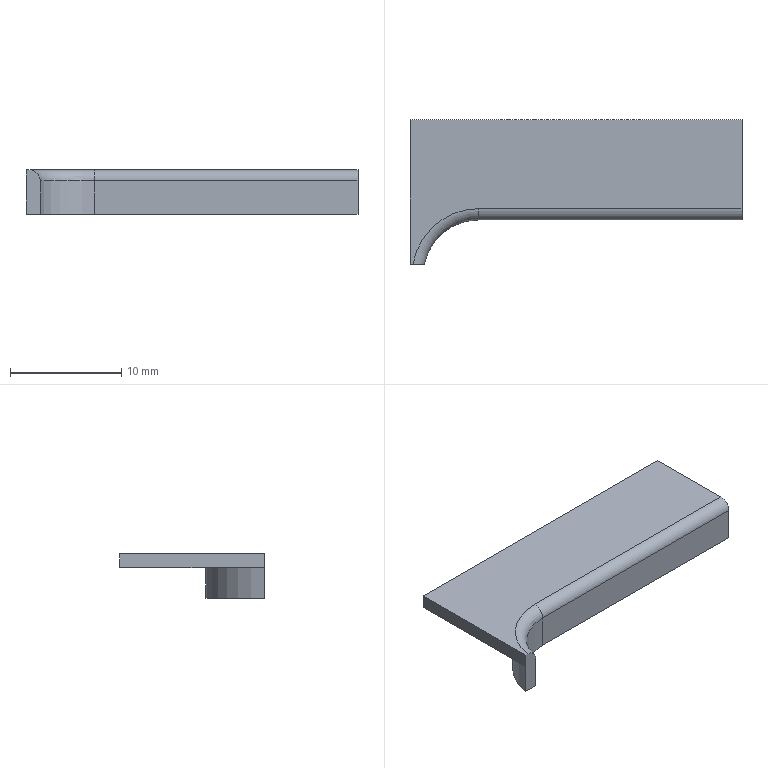Part | STEP file | gslz 2016.10.28-13_id970_x_t | 1 solid | 13 faces | box 29.791 x 13 x 4 mm | volume 449.169 mm3 | plane 9 | cylinder 3 | torus 1 | commonest cylinder face diameters 2 x1 10 x1 12.5 x1
STEP:
#1=CARTESIAN_POINT('',(0.,0.,0.));
#2=DIRECTION('',(0.,0.,1.));
#3=DIRECTION('',(1.,0.,0.));
#4=AXIS2_PLACEMENT_3D('',#1,#2,#3);
#5=CARTESIAN_POINT('',(-716.176,-264.75,0.));
#6=VERTEX_POINT('',#5);
#7=CARTESIAN_POINT('',(-722.345,-270.,0.));
#8=VERTEX_POINT('',#7);
#9=CARTESIAN_POINT('',(-716.176,-271.,0.));
#10=DIRECTION('',(0.,0.,1.));
#11=DIRECTION('',(1.,0.,0.));
#12=AXIS2_PLACEMENT_3D('',#9,#10,#11);
#13=CIRCLE('',#12,6.25);
#14=CARTESIAN_POINT('',(-716.176,-271.,0.625));
#15=DIRECTION('',(0.,0.,1.));
#16=DIRECTION('',(1.,0.,0.));
#17=AXIS2_PLACEMENT_3D('',#14,#15,#16);
#18=CYLINDRICAL_SURFACE('',#17,6.25);
#19=CARTESIAN_POINT('',(0.,-0.625));
#20=DIRECTION('',(1.,0.));
#21=VECTOR('',#20,1.);
#22=LINE('',#19,#21);
#23=(GEOMETRIC_REPRESENTATION_CONTEXT(2)PARAMETRIC_REPRESENTATION_CONTEXT()REPRESENTATION_CONTEXT('',''));
#24=DEFINITIONAL_REPRESENTATION('',(#22),#23);
#25=PCURVE('',#18,#24);
#26=CARTESIAN_POINT('',(1793.591,319.067,0.));
#27=DIRECTION('',(0.,0.,1.));
#28=DIRECTION('',(1.,0.,0.));
#29=AXIS2_PLACEMENT_3D('',#26,#27,#28);
#30=PLANE('',#29);
#31=CARTESIAN_POINT('',(-2509.767,-590.067));
#32=DIRECTION('',(1.,0.));
#33=AXIS2_PLACEMENT_2D('',#31,#32);
#34=CIRCLE('',#33,6.25);
#35=(GEOMETRIC_REPRESENTATION_CONTEXT(2)PARAMETRIC_REPRESENTATION_CONTEXT()REPRESENTATION_CONTEXT('',''));
#36=DEFINITIONAL_REPRESENTATION('',(#34),#35);
#37=PCURVE('',#30,#36);
#38=SURFACE_CURVE('',#13,(#25,#37),.PCURVE_S1.);
#39=EDGE_CURVE('',#6,#8,#38,.T.);
#40=ORIENTED_EDGE('',*,*,#39,.F.);
#41=CARTESIAN_POINT('',(-716.176,-264.75,-2.75));
#42=VERTEX_POINT('',#41);
#43=CARTESIAN_POINT('',(-716.176,-264.75,-0.75));
#44=DIRECTION('',(0.,0.,1.));
#45=VECTOR('',#44,1.);
#46=LINE('',#43,#45);
#47=CARTESIAN_POINT('',(1.571,-1.375));
#48=DIRECTION('',(0.,1.));
#49=VECTOR('',#48,1.);
#50=LINE('',#47,#49);
#51=(GEOMETRIC_REPRESENTATION_CONTEXT(2)PARAMETRIC_REPRESENTATION_CONTEXT()REPRESENTATION_CONTEXT('',''));
#52=DEFINITIONAL_REPRESENTATION('',(#50),#51);
#53=PCURVE('',#18,#52);
#54=CARTESIAN_POINT('',(1463.925,-264.75,-135.834));
#55=DIRECTION('',(0.,-1.,0.));
#56=DIRECTION('',(1.,0.,0.));
#57=AXIS2_PLACEMENT_3D('',#54,#55,#56);
#58=PLANE('',#57);
#59=CARTESIAN_POINT('',(-2180.101,135.084));
#60=DIRECTION('',(0.,1.));
#61=VECTOR('',#60,1.);
#62=LINE('',#59,#61);
#63=(GEOMETRIC_REPRESENTATION_CONTEXT(2)PARAMETRIC_REPRESENTATION_CONTEXT()REPRESENTATION_CONTEXT('',''));
#64=DEFINITIONAL_REPRESENTATION('',(#62),#63);
#65=PCURVE('',#58,#64);
#66=SURFACE_CURVE('',#46,(#53,#65),.PCURVE_S1.);
#67=EDGE_CURVE('',#42,#6,#66,.T.);
#68=ORIENTED_EDGE('',*,*,#67,.F.);
#69=CARTESIAN_POINT('',(-722.345,-270.,-2.75));
#70=VERTEX_POINT('',#69);
#71=CARTESIAN_POINT('',(-716.176,-271.,-2.75));
#72=DIRECTION('',(0.,0.,-1.));
#73=DIRECTION('',(1.,0.,0.));
#74=AXIS2_PLACEMENT_3D('',#71,#72,#73);
#75=CIRCLE('',#74,6.25);
#76=CARTESIAN_POINT('',(6.283,-3.375));
#77=DIRECTION('',(-1.,0.));
#78=VECTOR('',#77,1.);
#79=LINE('',#76,#78);
#80=(GEOMETRIC_REPRESENTATION_CONTEXT(2)PARAMETRIC_REPRESENTATION_CONTEXT()REPRESENTATION_CONTEXT('',''));
#81=DEFINITIONAL_REPRESENTATION('',(#79),#80);
#82=PCURVE('',#18,#81);
#83=CARTESIAN_POINT('',(-1810.,-266.,-2.75));
#84=DIRECTION('',(0.,0.,1.));
#85=DIRECTION('',(-1.,0.,0.));
#86=AXIS2_PLACEMENT_3D('',#83,#84,#85);
#87=PLANE('',#86);
#88=CARTESIAN_POINT('',(-1100.074,5.));
#89=CARTESIAN_POINT('',(-1100.074,15.825));
#90=CARTESIAN_POINT('',(-1090.699,10.413));
#91=CARTESIAN_POINT('',(-1081.324,5.));
#92=CARTESIAN_POINT('',(-1090.699,-0.4127));
#93=CARTESIAN_POINT('',(-1100.074,-5.825));
#94=CARTESIAN_POINT('',(-1100.074,5.));
#95=(BOUNDED_CURVE()B_SPLINE_CURVE(2,(#88,#89,#90,#91,#92,#93,#94),.UNSPECIFIED.,.T.,.F.)B_SPLINE_CURVE_WITH_KNOTS((1,2,2,2,2,1),(-2.094,0.,2.094,4.189,6.283,8.378),.UNSPECIFIED.)CURVE()GEOMETRIC_REPRESENTATION_ITEM()RATIONAL_B_SPLINE_CURVE((1.,0.5,1.,0.5,1.,0.5,1.))REPRESENTATION_ITEM(''));
#96=(GEOMETRIC_REPRESENTATION_CONTEXT(2)PARAMETRIC_REPRESENTATION_CONTEXT()REPRESENTATION_CONTEXT('',''));
#97=DEFINITIONAL_REPRESENTATION('',(#95),#96);
#98=PCURVE('',#87,#97);
#99=SURFACE_CURVE('',#75,(#82,#98),.PCURVE_S1.);
#100=EDGE_CURVE('',#70,#42,#99,.T.);
#101=ORIENTED_EDGE('',*,*,#100,.F.);
#102=CARTESIAN_POINT('',(-722.345,-270.,0.625));
#103=DIRECTION('',(0.,0.,-1.));
#104=VECTOR('',#103,1.);
#105=LINE('',#102,#104);
#106=CARTESIAN_POINT('',(2.981,0.));
#107=DIRECTION('',(0.,-1.));
#108=VECTOR('',#107,1.);
#109=LINE('',#106,#108);
#110=(GEOMETRIC_REPRESENTATION_CONTEXT(2)PARAMETRIC_REPRESENTATION_CONTEXT()REPRESENTATION_CONTEXT('',''));
#111=DEFINITIONAL_REPRESENTATION('',(#109),#110);
#112=PCURVE('',#18,#111);
#113=CARTESIAN_POINT('',(-1810.,-270.,1.25));
#114=DIRECTION('',(0.,1.,0.));
#115=DIRECTION('',(-1.,0.,0.));
#116=AXIS2_PLACEMENT_3D('',#113,#114,#115);
#117=PLANE('',#116);
#118=CARTESIAN_POINT('',(-1087.655,-0.625));
#119=DIRECTION('',(0.,-1.));
#120=VECTOR('',#119,1.);
#121=LINE('',#118,#120);
#122=(GEOMETRIC_REPRESENTATION_CONTEXT(2)PARAMETRIC_REPRESENTATION_CONTEXT()REPRESENTATION_CONTEXT('',''));
#123=DEFINITIONAL_REPRESENTATION('',(#121),#122);
#124=PCURVE('',#117,#123);
#125=SURFACE_CURVE('',#105,(#112,#124),.PCURVE_S1.);
#126=EDGE_CURVE('',#8,#70,#125,.T.);
#127=ORIENTED_EDGE('',*,*,#126,.F.);
#128=EDGE_LOOP('',(#40,#68,#101,#127));
#129=FACE_BOUND('',#128,.T.);
#130=ADVANCED_FACE('',(#129),#18,.T.);
#131=CARTESIAN_POINT('',(-721.075,-270.,-2.75));
#132=VERTEX_POINT('',#131);
#133=CARTESIAN_POINT('',(-721.075,-270.,0.25));
#134=VERTEX_POINT('',#133);
#135=CARTESIAN_POINT('',(-721.075,-270.,61.25));
#136=DIRECTION('',(0.,0.,1.));
#137=VECTOR('',#136,1.);
#138=LINE('',#135,#137);
#139=CARTESIAN_POINT('',(-1088.925,60.));
#140=DIRECTION('',(0.,1.));
#141=VECTOR('',#140,1.);
#142=LINE('',#139,#141);
#143=(GEOMETRIC_REPRESENTATION_CONTEXT(2)PARAMETRIC_REPRESENTATION_CONTEXT()REPRESENTATION_CONTEXT('',''));
#144=DEFINITIONAL_REPRESENTATION('',(#142),#143);
#145=PCURVE('',#117,#144);
#146=CARTESIAN_POINT('',(-716.176,-271.,61.25));
#147=DIRECTION('',(0.,0.,-1.));
#148=DIRECTION('',(-1.,0.,0.));
#149=AXIS2_PLACEMENT_3D('',#146,#147,#148);
#150=CYLINDRICAL_SURFACE('',#149,5.);
#151=CARTESIAN_POINT('',(0.2014,0.));
#152=DIRECTION('',(0.,-1.));
#153=VECTOR('',#152,1.);
#154=LINE('',#151,#153);
#155=(GEOMETRIC_REPRESENTATION_CONTEXT(2)PARAMETRIC_REPRESENTATION_CONTEXT()REPRESENTATION_CONTEXT('',''));
#156=DEFINITIONAL_REPRESENTATION('',(#154),#155);
#157=PCURVE('',#150,#156);
#158=SURFACE_CURVE('',#138,(#145,#157),.PCURVE_S1.);
#159=EDGE_CURVE('',#132,#134,#158,.T.);
#160=ORIENTED_EDGE('',*,*,#159,.T.);
#161=CARTESIAN_POINT('',(-722.092,-270.,1.25));
#162=VERTEX_POINT('',#161);
#163=CARTESIAN_POINT('',(-721.075,-270.,0.25));
#164=CARTESIAN_POINT('',(-721.075,-270.,0.3603));
#165=CARTESIAN_POINT('',(-721.094,-270.,0.4722));
#166=CARTESIAN_POINT('',(-721.131,-270.,0.5763));
#167=CARTESIAN_POINT('',(-721.167,-270.,0.6803));
#168=CARTESIAN_POINT('',(-721.222,-270.,0.7794));
#169=CARTESIAN_POINT('',(-721.291,-270.,0.8657));
#170=CARTESIAN_POINT('',(-721.36,-270.,0.9528));
#171=CARTESIAN_POINT('',(-721.445,-270.,1.029));
#172=CARTESIAN_POINT('',(-721.539,-270.,1.089));
#173=CARTESIAN_POINT('',(-721.635,-270.,1.15));
#174=CARTESIAN_POINT('',(-721.742,-270.,1.196));
#175=CARTESIAN_POINT('',(-721.853,-270.,1.222));
#176=CARTESIAN_POINT('',(-721.931,-270.,1.24));
#177=CARTESIAN_POINT('',(-722.012,-270.,1.25));
#178=CARTESIAN_POINT('',(-722.092,-270.,1.25));
#179=B_SPLINE_CURVE_WITH_KNOTS('',3,(#163,#164,#165,#166,#167,#168,#169,#170,#171,#172,#173,#174,#175,#176,#177,#178),.UNSPECIFIED.,.F.,.F.,(4,3,3,3,3,4),(0.,0.2101,0.4202,0.6322,0.8483,1.),.UNSPECIFIED.);
#180=CARTESIAN_POINT('',(-1088.925,-1.));
#181=CARTESIAN_POINT('',(-1088.925,-0.8897));
#182=CARTESIAN_POINT('',(-1088.906,-0.7778));
#183=CARTESIAN_POINT('',(-1088.869,-0.6737));
#184=CARTESIAN_POINT('',(-1088.833,-0.5697));
#185=CARTESIAN_POINT('',(-1088.778,-0.4706));
#186=CARTESIAN_POINT('',(-1088.709,-0.3843));
#187=CARTESIAN_POINT('',(-1088.64,-0.2972));
#188=CARTESIAN_POINT('',(-1088.555,-0.2207));
#189=CARTESIAN_POINT('',(-1088.461,-0.1609));
#190=CARTESIAN_POINT('',(-1088.365,-0.0999));
#191=CARTESIAN_POINT('',(-1088.258,-0.05448));
#192=CARTESIAN_POINT('',(-1088.147,-0.02814));
#193=CARTESIAN_POINT('',(-1088.069,-0.009512));
#194=CARTESIAN_POINT('',(-1087.988,0.));
#195=CARTESIAN_POINT('',(-1087.908,0.));
#196=B_SPLINE_CURVE_WITH_KNOTS('',3,(#180,#181,#182,#183,#184,#185,#186,#187,#188,#189,#190,#191,#192,#193,#194,#195),.UNSPECIFIED.,.F.,.F.,(4,3,3,3,3,4),(0.,0.2101,0.4202,0.6322,0.8483,1.),.UNSPECIFIED.);
#197=(GEOMETRIC_REPRESENTATION_CONTEXT(2)PARAMETRIC_REPRESENTATION_CONTEXT()REPRESENTATION_CONTEXT('',''));
#198=DEFINITIONAL_REPRESENTATION('',(#196),#197);
#199=PCURVE('',#117,#198);
#200=CARTESIAN_POINT('',(-716.176,-271.,0.25));
#201=DIRECTION('',(0.,0.,1.));
#202=DIRECTION('',(1.,0.,0.));
#203=AXIS2_PLACEMENT_3D('',#200,#201,#202);
#204=TOROIDAL_SURFACE('',#203,6.,1.);
#205=CARTESIAN_POINT('',(2.94,3.142));
#206=CARTESIAN_POINT('',(2.974,1.571));
#207=B_SPLINE_CURVE_WITH_KNOTS('',1,(#205,#206),.UNSPECIFIED.,.F.,.F.,(2,2),(0.,1.),.PIECEWISE_BEZIER_KNOTS.);
#208=(GEOMETRIC_REPRESENTATION_CONTEXT(2)PARAMETRIC_REPRESENTATION_CONTEXT()REPRESENTATION_CONTEXT('',''));
#209=DEFINITIONAL_REPRESENTATION('',(#207),#208);
#210=PCURVE('',#204,#209);
#211=SURFACE_CURVE('',#179,(#199,#210),.PCURVE_S1.);
#212=EDGE_CURVE('',#134,#162,#211,.T.);
#213=ORIENTED_EDGE('',*,*,#212,.T.);
#214=CARTESIAN_POINT('',(-722.345,-270.,1.25));
#215=VERTEX_POINT('',#214);
#216=CARTESIAN_POINT('',(-1810.,-270.,1.25));
#217=DIRECTION('',(-1.,0.,0.));
#218=VECTOR('',#217,1.);
#219=LINE('',#216,#218);
#220=CARTESIAN_POINT('',(0.,0.));
#221=DIRECTION('',(1.,0.));
#222=VECTOR('',#221,1.);
#223=LINE('',#220,#222);
#224=(GEOMETRIC_REPRESENTATION_CONTEXT(2)PARAMETRIC_REPRESENTATION_CONTEXT()REPRESENTATION_CONTEXT('',''));
#225=DEFINITIONAL_REPRESENTATION('',(#223),#224);
#226=PCURVE('',#117,#225);
#227=CARTESIAN_POINT('',(1793.591,319.067,1.25));
#228=DIRECTION('',(0.,0.,1.));
#229=DIRECTION('',(1.,0.,0.));
#230=AXIS2_PLACEMENT_3D('',#227,#228,#229);
#231=PLANE('',#230);
#232=CARTESIAN_POINT('',(-3603.591,-589.067));
#233=DIRECTION('',(-1.,0.));
#234=VECTOR('',#233,1.);
#235=LINE('',#232,#234);
#236=(GEOMETRIC_REPRESENTATION_CONTEXT(2)PARAMETRIC_REPRESENTATION_CONTEXT()REPRESENTATION_CONTEXT('',''));
#237=DEFINITIONAL_REPRESENTATION('',(#235),#236);
#238=PCURVE('',#231,#237);
#239=SURFACE_CURVE('',#219,(#226,#238),.PCURVE_S1.);
#240=EDGE_CURVE('',#162,#215,#239,.T.);
#241=ORIENTED_EDGE('',*,*,#240,.T.);
#242=CARTESIAN_POINT('',(-722.345,-270.,0.625));
#243=DIRECTION('',(0.,0.,-1.));
#244=VECTOR('',#243,1.);
#245=LINE('',#242,#244);
#246=CARTESIAN_POINT('',(-1087.655,-0.625));
#247=DIRECTION('',(0.,-1.));
#248=VECTOR('',#247,1.);
#249=LINE('',#246,#248);
#250=(GEOMETRIC_REPRESENTATION_CONTEXT(2)PARAMETRIC_REPRESENTATION_CONTEXT()REPRESENTATION_CONTEXT('',''));
#251=DEFINITIONAL_REPRESENTATION('',(#249),#250);
#252=PCURVE('',#117,#251);
#253=CARTESIAN_POINT('',(-722.345,-275.25,-0.75));
#254=DIRECTION('',(-1.,0.,0.));
#255=DIRECTION('',(0.,-1.,0.));
#256=AXIS2_PLACEMENT_3D('',#253,#254,#255);
#257=PLANE('',#256);
#258=CARTESIAN_POINT('',(-5.25,1.375));
#259=DIRECTION('',(0.,-1.));
#260=VECTOR('',#259,1.);
#261=LINE('',#258,#260);
#262=(GEOMETRIC_REPRESENTATION_CONTEXT(2)PARAMETRIC_REPRESENTATION_CONTEXT()REPRESENTATION_CONTEXT('',''));
#263=DEFINITIONAL_REPRESENTATION('',(#261),#262);
#264=PCURVE('',#257,#263);
#265=SURFACE_CURVE('',#245,(#252,#264),.PCURVE_S1.);
#266=EDGE_CURVE('',#215,#8,#265,.T.);
#267=ORIENTED_EDGE('',*,*,#266,.T.);
#268=ORIENTED_EDGE('',*,*,#126,.T.);
#269=CARTESIAN_POINT('',(-1810.,-270.,-2.75));
#270=DIRECTION('',(1.,0.,0.));
#271=VECTOR('',#270,1.);
#272=LINE('',#269,#271);
#273=CARTESIAN_POINT('',(0.,-4.));
#274=DIRECTION('',(-1.,0.));
#275=VECTOR('',#274,1.);
#276=LINE('',#273,#275);
#277=(GEOMETRIC_REPRESENTATION_CONTEXT(2)PARAMETRIC_REPRESENTATION_CONTEXT()REPRESENTATION_CONTEXT('',''));
#278=DEFINITIONAL_REPRESENTATION('',(#276),#277);
#279=PCURVE('',#117,#278);
#280=CARTESIAN_POINT('',(0.,4.));
#281=DIRECTION('',(-1.,0.));
#282=VECTOR('',#281,1.);
#283=LINE('',#280,#282);
#284=(GEOMETRIC_REPRESENTATION_CONTEXT(2)PARAMETRIC_REPRESENTATION_CONTEXT()REPRESENTATION_CONTEXT('',''));
#285=DEFINITIONAL_REPRESENTATION('',(#283),#284);
#286=PCURVE('',#87,#285);
#287=SURFACE_CURVE('',#272,(#279,#286),.PCURVE_S1.);
#288=EDGE_CURVE('',#70,#132,#287,.T.);
#289=ORIENTED_EDGE('',*,*,#288,.T.);
#290=EDGE_LOOP('',(#160,#213,#241,#267,#268,#289));
#291=FACE_BOUND('',#290,.T.);
#292=ADVANCED_FACE('',(#291),#117,.F.);
#293=CARTESIAN_POINT('',(-716.176,-266.,-2.75));
#294=VERTEX_POINT('',#293);
#295=CARTESIAN_POINT('',(-716.176,-271.,-2.75));
#296=DIRECTION('',(0.,0.,1.));
#297=DIRECTION('',(1.,0.,0.));
#298=AXIS2_PLACEMENT_3D('',#295,#296,#297);
#299=CIRCLE('',#298,5.);
#300=CARTESIAN_POINT('',(3.142,64.));
#301=DIRECTION('',(-1.,0.));
#302=VECTOR('',#301,1.);
#303=LINE('',#300,#302);
#304=(GEOMETRIC_REPRESENTATION_CONTEXT(2)PARAMETRIC_REPRESENTATION_CONTEXT()REPRESENTATION_CONTEXT('',''));
#305=DEFINITIONAL_REPRESENTATION('',(#303),#304);
#306=PCURVE('',#150,#305);
#307=CARTESIAN_POINT('',(-1093.824,5.));
#308=DIRECTION('',(-1.,0.));
#309=AXIS2_PLACEMENT_2D('',#307,#308);
#310=CIRCLE('',#309,5.);
#311=(GEOMETRIC_REPRESENTATION_CONTEXT(2)PARAMETRIC_REPRESENTATION_CONTEXT()REPRESENTATION_CONTEXT('',''));
#312=DEFINITIONAL_REPRESENTATION('',(#310),#311);
#313=PCURVE('',#87,#312);
#314=SURFACE_CURVE('',#299,(#306,#313),.PCURVE_S1.);
#315=EDGE_CURVE('',#294,#132,#314,.T.);
#316=ORIENTED_EDGE('',*,*,#315,.T.);
#317=ORIENTED_EDGE('',*,*,#159,.T.);
#318=CARTESIAN_POINT('',(-716.176,-266.,0.25));
#319=VERTEX_POINT('',#318);
#320=CARTESIAN_POINT('',(-716.176,-271.,0.25));
#321=DIRECTION('',(0.,0.,1.));
#322=DIRECTION('',(1.,0.,0.));
#323=AXIS2_PLACEMENT_3D('',#320,#321,#322);
#324=CIRCLE('',#323,5.);
#325=CARTESIAN_POINT('',(3.142,61.));
#326=DIRECTION('',(-1.,0.));
#327=VECTOR('',#326,1.);
#328=LINE('',#325,#327);
#329=(GEOMETRIC_REPRESENTATION_CONTEXT(2)PARAMETRIC_REPRESENTATION_CONTEXT()REPRESENTATION_CONTEXT('',''));
#330=DEFINITIONAL_REPRESENTATION('',(#328),#329);
#331=PCURVE('',#150,#330);
#332=CARTESIAN_POINT('',(0.,3.142));
#333=DIRECTION('',(1.,0.));
#334=VECTOR('',#333,1.);
#335=LINE('',#332,#334);
#336=(GEOMETRIC_REPRESENTATION_CONTEXT(2)PARAMETRIC_REPRESENTATION_CONTEXT()REPRESENTATION_CONTEXT('',''));
#337=DEFINITIONAL_REPRESENTATION('',(#335),#336);
#338=PCURVE('',#204,#337);
#339=SURFACE_CURVE('',#324,(#331,#338),.PCURVE_S1.);
#340=EDGE_CURVE('',#319,#134,#339,.T.);
#341=ORIENTED_EDGE('',*,*,#340,.F.);
#342=CARTESIAN_POINT('',(-716.176,-266.,61.25));
#343=DIRECTION('',(0.,0.,-1.));
#344=VECTOR('',#343,1.);
#345=LINE('',#342,#344);
#346=CARTESIAN_POINT('',(1.571,0.));
#347=DIRECTION('',(0.,1.));
#348=VECTOR('',#347,1.);
#349=LINE('',#346,#348);
#350=(GEOMETRIC_REPRESENTATION_CONTEXT(2)PARAMETRIC_REPRESENTATION_CONTEXT()REPRESENTATION_CONTEXT('',''));
#351=DEFINITIONAL_REPRESENTATION('',(#349),#350);
#352=PCURVE('',#150,#351);
#353=CARTESIAN_POINT('',(-548.575,-266.,0.625));
#354=DIRECTION('',(0.,-1.,0.));
#355=DIRECTION('',(1.,0.,0.));
#356=AXIS2_PLACEMENT_3D('',#353,#354,#355);
#357=PLANE('',#356);
#358=CARTESIAN_POINT('',(-167.601,60.625));
#359=DIRECTION('',(0.,-1.));
#360=VECTOR('',#359,1.);
#361=LINE('',#358,#360);
#362=(GEOMETRIC_REPRESENTATION_CONTEXT(2)PARAMETRIC_REPRESENTATION_CONTEXT()REPRESENTATION_CONTEXT('',''));
#363=DEFINITIONAL_REPRESENTATION('',(#361),#362);
#364=PCURVE('',#357,#363);
#365=SURFACE_CURVE('',#345,(#352,#364),.PCURVE_S1.);
#366=EDGE_CURVE('',#319,#294,#365,.T.);
#367=ORIENTED_EDGE('',*,*,#366,.T.);
#368=EDGE_LOOP('',(#316,#317,#341,#367));
#369=FACE_BOUND('',#368,.F.);
#370=ADVANCED_FACE('',(#369),#150,.F.);
#371=ORIENTED_EDGE('',*,*,#212,.F.);
#372=ORIENTED_EDGE('',*,*,#340,.F.);
#373=CARTESIAN_POINT('',(-716.176,-265.,1.25));
#374=VERTEX_POINT('',#373);
#375=CARTESIAN_POINT('',(-716.176,-265.,0.25));
#376=DIRECTION('',(1.,0.,0.));
#377=DIRECTION('',(0.,0.,-1.));
#378=AXIS2_PLACEMENT_3D('',#375,#376,#377);
#379=CIRCLE('',#378,1.);
#380=CARTESIAN_POINT('',(1.571,-1.571));
#381=DIRECTION('',(0.,1.));
#382=VECTOR('',#381,1.);
#383=LINE('',#380,#382);
#384=(GEOMETRIC_REPRESENTATION_CONTEXT(2)PARAMETRIC_REPRESENTATION_CONTEXT()REPRESENTATION_CONTEXT('',''));
#385=DEFINITIONAL_REPRESENTATION('',(#383),#384);
#386=PCURVE('',#204,#385);
#387=CARTESIAN_POINT('',(1793.591,-265.,0.25));
#388=DIRECTION('',(1.,0.,0.));
#389=DIRECTION('',(0.,1.,0.));
#390=AXIS2_PLACEMENT_3D('',#387,#388,#389);
#391=CYLINDRICAL_SURFACE('',#390,1.);
#392=CARTESIAN_POINT('',(-1.571,-2509.767));
#393=DIRECTION('',(1.,0.));
#394=VECTOR('',#393,1.);
#395=LINE('',#392,#394);
#396=(GEOMETRIC_REPRESENTATION_CONTEXT(2)PARAMETRIC_REPRESENTATION_CONTEXT()REPRESENTATION_CONTEXT('',''));
#397=DEFINITIONAL_REPRESENTATION('',(#395),#396);
#398=PCURVE('',#391,#397);
#399=SURFACE_CURVE('',#379,(#386,#398),.PCURVE_S1.);
#400=EDGE_CURVE('',#374,#319,#399,.T.);
#401=ORIENTED_EDGE('',*,*,#400,.F.);
#402=CARTESIAN_POINT('',(-716.176,-271.,1.25));
#403=DIRECTION('',(0.,0.,-1.));
#404=DIRECTION('',(1.,0.,0.));
#405=AXIS2_PLACEMENT_3D('',#402,#403,#404);
#406=CIRCLE('',#405,6.);
#407=CARTESIAN_POINT('',(6.283,1.571));
#408=DIRECTION('',(-1.,0.));
#409=VECTOR('',#408,1.);
#410=LINE('',#407,#409);
#411=(GEOMETRIC_REPRESENTATION_CONTEXT(2)PARAMETRIC_REPRESENTATION_CONTEXT()REPRESENTATION_CONTEXT('',''));
#412=DEFINITIONAL_REPRESENTATION('',(#410),#411);
#413=PCURVE('',#204,#412);
#414=CARTESIAN_POINT('',(-2503.767,-590.067));
#415=CARTESIAN_POINT('',(-2503.767,-600.459));
#416=CARTESIAN_POINT('',(-2512.767,-595.263));
#417=CARTESIAN_POINT('',(-2521.767,-590.067));
#418=CARTESIAN_POINT('',(-2512.767,-584.871));
#419=CARTESIAN_POINT('',(-2503.767,-579.674));
#420=CARTESIAN_POINT('',(-2503.767,-590.067));
#421=(BOUNDED_CURVE()B_SPLINE_CURVE(2,(#414,#415,#416,#417,#418,#419,#420),.UNSPECIFIED.,.T.,.F.)B_SPLINE_CURVE_WITH_KNOTS((1,2,2,2,2,1),(-2.094,0.,2.094,4.189,6.283,8.378),.UNSPECIFIED.)CURVE()GEOMETRIC_REPRESENTATION_ITEM()RATIONAL_B_SPLINE_CURVE((1.,0.5,1.,0.5,1.,0.5,1.))REPRESENTATION_ITEM(''));
#422=(GEOMETRIC_REPRESENTATION_CONTEXT(2)PARAMETRIC_REPRESENTATION_CONTEXT()REPRESENTATION_CONTEXT('',''));
#423=DEFINITIONAL_REPRESENTATION('',(#421),#422);
#424=PCURVE('',#231,#423);
#425=SURFACE_CURVE('',#406,(#413,#424),.PCURVE_S1.);
#426=EDGE_CURVE('',#162,#374,#425,.T.);
#427=ORIENTED_EDGE('',*,*,#426,.F.);
#428=EDGE_LOOP('',(#371,#372,#401,#427));
#429=FACE_BOUND('',#428,.T.);
#430=ADVANCED_FACE('',(#429),#204,.T.);
#431=CARTESIAN_POINT('',(-722.345,-257.,1.25));
#432=VERTEX_POINT('',#431);
#433=CARTESIAN_POINT('',(-722.345,319.067,1.25));
#434=DIRECTION('',(0.,1.,0.));
#435=VECTOR('',#434,1.);
#436=LINE('',#433,#435);
#437=CARTESIAN_POINT('',(-594.317,2.));
#438=DIRECTION('',(-1.,0.));
#439=VECTOR('',#438,1.);
#440=LINE('',#437,#439);
#441=(GEOMETRIC_REPRESENTATION_CONTEXT(2)PARAMETRIC_REPRESENTATION_CONTEXT()REPRESENTATION_CONTEXT('',''));
#442=DEFINITIONAL_REPRESENTATION('',(#440),#441);
#443=PCURVE('',#257,#442);
#444=CARTESIAN_POINT('',(-2515.936,0.));
#445=DIRECTION('',(0.,1.));
#446=VECTOR('',#445,1.);
#447=LINE('',#444,#446);
#448=(GEOMETRIC_REPRESENTATION_CONTEXT(2)PARAMETRIC_REPRESENTATION_CONTEXT()REPRESENTATION_CONTEXT('',''));
#449=DEFINITIONAL_REPRESENTATION('',(#447),#448);
#450=PCURVE('',#231,#449);
#451=SURFACE_CURVE('',#436,(#443,#450),.PCURVE_S1.);
#452=EDGE_CURVE('',#215,#432,#451,.T.);
#453=ORIENTED_EDGE('',*,*,#452,.T.);
#454=CARTESIAN_POINT('',(-722.345,-257.,0.));
#455=VERTEX_POINT('',#454);
#456=CARTESIAN_POINT('',(-722.345,-257.,2.5));
#457=DIRECTION('',(0.,0.,1.));
#458=VECTOR('',#457,1.);
#459=LINE('',#456,#458);
#460=CARTESIAN_POINT('',(-18.25,3.25));
#461=DIRECTION('',(0.,1.));
#462=VECTOR('',#461,1.);
#463=LINE('',#460,#462);
#464=(GEOMETRIC_REPRESENTATION_CONTEXT(2)PARAMETRIC_REPRESENTATION_CONTEXT()REPRESENTATION_CONTEXT('',''));
#465=DEFINITIONAL_REPRESENTATION('',(#463),#464);
#466=PCURVE('',#257,#465);
#467=CARTESIAN_POINT('',(-705.557,-257.,2.5));
#468=DIRECTION('',(0.,1.,0.));
#469=DIRECTION('',(0.,0.,1.));
#470=AXIS2_PLACEMENT_3D('',#467,#468,#469);
#471=PLANE('',#470);
#472=CARTESIAN_POINT('',(0.,-16.788));
#473=DIRECTION('',(1.,0.));
#474=VECTOR('',#473,1.);
#475=LINE('',#472,#474);
#476=(GEOMETRIC_REPRESENTATION_CONTEXT(2)PARAMETRIC_REPRESENTATION_CONTEXT()REPRESENTATION_CONTEXT('',''));
#477=DEFINITIONAL_REPRESENTATION('',(#475),#476);
#478=PCURVE('',#471,#477);
#479=SURFACE_CURVE('',#459,(#466,#478),.PCURVE_S1.);
#480=EDGE_CURVE('',#455,#432,#479,.T.);
#481=ORIENTED_EDGE('',*,*,#480,.F.);
#482=CARTESIAN_POINT('',(-722.345,319.067,0.));
#483=DIRECTION('',(0.,1.,0.));
#484=VECTOR('',#483,1.);
#485=LINE('',#482,#484);
#486=CARTESIAN_POINT('',(-594.317,0.75));
#487=DIRECTION('',(-1.,0.));
#488=VECTOR('',#487,1.);
#489=LINE('',#486,#488);
#490=(GEOMETRIC_REPRESENTATION_CONTEXT(2)PARAMETRIC_REPRESENTATION_CONTEXT()REPRESENTATION_CONTEXT('',''));
#491=DEFINITIONAL_REPRESENTATION('',(#489),#490);
#492=PCURVE('',#257,#491);
#493=CARTESIAN_POINT('',(-2515.936,0.));
#494=DIRECTION('',(0.,1.));
#495=VECTOR('',#494,1.);
#496=LINE('',#493,#495);
#497=(GEOMETRIC_REPRESENTATION_CONTEXT(2)PARAMETRIC_REPRESENTATION_CONTEXT()REPRESENTATION_CONTEXT('',''));
#498=DEFINITIONAL_REPRESENTATION('',(#496),#497);
#499=PCURVE('',#30,#498);
#500=SURFACE_CURVE('',#485,(#492,#499),.PCURVE_S1.);
#501=EDGE_CURVE('',#8,#455,#500,.T.);
#502=ORIENTED_EDGE('',*,*,#501,.F.);
#503=ORIENTED_EDGE('',*,*,#266,.F.);
#504=EDGE_LOOP('',(#453,#481,#502,#503));
#505=FACE_BOUND('',#504,.T.);
#506=ADVANCED_FACE('',(#505),#257,.T.);
#507=CARTESIAN_POINT('',(-692.554,-266.,0.25));
#508=VERTEX_POINT('',#507);
#509=CARTESIAN_POINT('',(-692.554,-265.,1.25));
#510=VERTEX_POINT('',#509);
#511=CARTESIAN_POINT('',(-692.554,-265.,0.25));
#512=DIRECTION('',(-1.,0.,0.));
#513=DIRECTION('',(0.,0.,1.));
#514=AXIS2_PLACEMENT_3D('',#511,#512,#513);
#515=CIRCLE('',#514,1.);
#516=CARTESIAN_POINT('',(7.854,-2486.145));
#517=DIRECTION('',(-1.,0.));
#518=VECTOR('',#517,1.);
#519=LINE('',#516,#518);
#520=(GEOMETRIC_REPRESENTATION_CONTEXT(2)PARAMETRIC_REPRESENTATION_CONTEXT()REPRESENTATION_CONTEXT('',''));
#521=DEFINITIONAL_REPRESENTATION('',(#519),#520);
#522=PCURVE('',#391,#521);
#523=CARTESIAN_POINT('',(-692.554,-244.358,-2.25));
#524=DIRECTION('',(-1.,0.,0.));
#525=DIRECTION('',(0.,0.,1.));
#526=AXIS2_PLACEMENT_3D('',#523,#524,#525);
#527=PLANE('',#526);
#528=CARTESIAN_POINT('',(2.5,-20.642));
#529=DIRECTION('',(1.,0.));
#530=AXIS2_PLACEMENT_2D('',#528,#529);
#531=CIRCLE('',#530,1.);
#532=(GEOMETRIC_REPRESENTATION_CONTEXT(2)PARAMETRIC_REPRESENTATION_CONTEXT()REPRESENTATION_CONTEXT('',''));
#533=DEFINITIONAL_REPRESENTATION('',(#531),#532);
#534=PCURVE('',#527,#533);
#535=SURFACE_CURVE('',#515,(#522,#534),.PCURVE_S1.);
#536=EDGE_CURVE('',#508,#510,#535,.T.);
#537=ORIENTED_EDGE('',*,*,#536,.T.);
#538=CARTESIAN_POINT('',(1793.591,-265.,1.25));
#539=DIRECTION('',(1.,0.,0.));
#540=VECTOR('',#539,1.);
#541=LINE('',#538,#540);
#542=CARTESIAN_POINT('',(1.571,0.));
#543=DIRECTION('',(0.,1.));
#544=VECTOR('',#543,1.);
#545=LINE('',#542,#544);
#546=(GEOMETRIC_REPRESENTATION_CONTEXT(2)PARAMETRIC_REPRESENTATION_CONTEXT()REPRESENTATION_CONTEXT('',''));
#547=DEFINITIONAL_REPRESENTATION('',(#545),#546);
#548=PCURVE('',#391,#547);
#549=CARTESIAN_POINT('',(0.,-584.067));
#550=DIRECTION('',(1.,0.));
#551=VECTOR('',#550,1.);
#552=LINE('',#549,#551);
#553=(GEOMETRIC_REPRESENTATION_CONTEXT(2)PARAMETRIC_REPRESENTATION_CONTEXT()REPRESENTATION_CONTEXT('',''));
#554=DEFINITIONAL_REPRESENTATION('',(#552),#553);
#555=PCURVE('',#231,#554);
#556=SURFACE_CURVE('',#541,(#548,#555),.PCURVE_S1.);
#557=EDGE_CURVE('',#374,#510,#556,.T.);
#558=ORIENTED_EDGE('',*,*,#557,.F.);
#559=ORIENTED_EDGE('',*,*,#400,.T.);
#560=CARTESIAN_POINT('',(-548.575,-266.,0.25));
#561=DIRECTION('',(-1.,0.,0.));
#562=VECTOR('',#561,1.);
#563=LINE('',#560,#562);
#564=CARTESIAN_POINT('',(3.142,-2342.166));
#565=DIRECTION('',(0.,-1.));
#566=VECTOR('',#565,1.);
#567=LINE('',#564,#566);
#568=(GEOMETRIC_REPRESENTATION_CONTEXT(2)PARAMETRIC_REPRESENTATION_CONTEXT()REPRESENTATION_CONTEXT('',''));
#569=DEFINITIONAL_REPRESENTATION('',(#567),#568);
#570=PCURVE('',#391,#569);
#571=CARTESIAN_POINT('',(0.,-0.375));
#572=DIRECTION('',(-1.,0.));
#573=VECTOR('',#572,1.);
#574=LINE('',#571,#573);
#575=(GEOMETRIC_REPRESENTATION_CONTEXT(2)PARAMETRIC_REPRESENTATION_CONTEXT()REPRESENTATION_CONTEXT('',''));
#576=DEFINITIONAL_REPRESENTATION('',(#574),#575);
#577=PCURVE('',#357,#576);
#578=SURFACE_CURVE('',#563,(#570,#577),.PCURVE_S1.);
#579=EDGE_CURVE('',#508,#319,#578,.T.);
#580=ORIENTED_EDGE('',*,*,#579,.F.);
#581=EDGE_LOOP('',(#537,#558,#559,#580));
#582=FACE_BOUND('',#581,.T.);
#583=ADVANCED_FACE('',(#582),#391,.T.);
#584=CARTESIAN_POINT('',(-692.554,-266.,-2.75));
#585=VERTEX_POINT('',#584);
#586=CARTESIAN_POINT('',(-692.554,-266.,0.625));
#587=DIRECTION('',(0.,0.,1.));
#588=VECTOR('',#587,1.);
#589=LINE('',#586,#588);
#590=CARTESIAN_POINT('',(-143.979,0.));
#591=DIRECTION('',(0.,1.));
#592=VECTOR('',#591,1.);
#593=LINE('',#590,#592);
#594=(GEOMETRIC_REPRESENTATION_CONTEXT(2)PARAMETRIC_REPRESENTATION_CONTEXT()REPRESENTATION_CONTEXT('',''));
#595=DEFINITIONAL_REPRESENTATION('',(#593),#594);
#596=PCURVE('',#357,#595);
#597=CARTESIAN_POINT('',(2.875,-21.642));
#598=DIRECTION('',(1.,0.));
#599=VECTOR('',#598,1.);
#600=LINE('',#597,#599);
#601=(GEOMETRIC_REPRESENTATION_CONTEXT(2)PARAMETRIC_REPRESENTATION_CONTEXT()REPRESENTATION_CONTEXT('',''));
#602=DEFINITIONAL_REPRESENTATION('',(#600),#601);
#603=PCURVE('',#527,#602);
#604=SURFACE_CURVE('',#589,(#596,#603),.PCURVE_S1.);
#605=EDGE_CURVE('',#585,#508,#604,.T.);
#606=ORIENTED_EDGE('',*,*,#605,.T.);
#607=ORIENTED_EDGE('',*,*,#579,.T.);
#608=ORIENTED_EDGE('',*,*,#366,.T.);
#609=CARTESIAN_POINT('',(-1810.,-266.,-2.75));
#610=DIRECTION('',(-1.,0.,0.));
#611=VECTOR('',#610,1.);
#612=LINE('',#609,#611);
#613=CARTESIAN_POINT('',(-1261.425,-3.375));
#614=DIRECTION('',(-1.,0.));
#615=VECTOR('',#614,1.);
#616=LINE('',#613,#615);
#617=(GEOMETRIC_REPRESENTATION_CONTEXT(2)PARAMETRIC_REPRESENTATION_CONTEXT()REPRESENTATION_CONTEXT('',''));
#618=DEFINITIONAL_REPRESENTATION('',(#616),#617);
#619=PCURVE('',#357,#618);
#620=CARTESIAN_POINT('',(0.,0.));
#621=DIRECTION('',(1.,0.));
#622=VECTOR('',#621,1.);
#623=LINE('',#620,#622);
#624=(GEOMETRIC_REPRESENTATION_CONTEXT(2)PARAMETRIC_REPRESENTATION_CONTEXT()REPRESENTATION_CONTEXT('',''));
#625=DEFINITIONAL_REPRESENTATION('',(#623),#624);
#626=PCURVE('',#87,#625);
#627=SURFACE_CURVE('',#612,(#619,#626),.PCURVE_S1.);
#628=EDGE_CURVE('',#585,#294,#627,.T.);
#629=ORIENTED_EDGE('',*,*,#628,.F.);
#630=EDGE_LOOP('',(#606,#607,#608,#629));
#631=FACE_BOUND('',#630,.T.);
#632=ADVANCED_FACE('',(#631),#357,.T.);
#633=CARTESIAN_POINT('',(-692.554,-264.75,-2.75));
#634=VERTEX_POINT('',#633);
#635=CARTESIAN_POINT('',(-1810.,-264.75,-2.75));
#636=DIRECTION('',(-1.,0.,0.));
#637=VECTOR('',#636,1.);
#638=LINE('',#635,#637);
#639=CARTESIAN_POINT('',(0.,-1.25));
#640=DIRECTION('',(1.,0.));
#641=VECTOR('',#640,1.);
#642=LINE('',#639,#641);
#643=(GEOMETRIC_REPRESENTATION_CONTEXT(2)PARAMETRIC_REPRESENTATION_CONTEXT()REPRESENTATION_CONTEXT('',''));
#644=DEFINITIONAL_REPRESENTATION('',(#642),#643);
#645=PCURVE('',#87,#644);
#646=CARTESIAN_POINT('',(-3273.925,133.084));
#647=DIRECTION('',(-1.,0.));
#648=VECTOR('',#647,1.);
#649=LINE('',#646,#648);
#650=(GEOMETRIC_REPRESENTATION_CONTEXT(2)PARAMETRIC_REPRESENTATION_CONTEXT()REPRESENTATION_CONTEXT('',''));
#651=DEFINITIONAL_REPRESENTATION('',(#649),#650);
#652=PCURVE('',#58,#651);
#653=SURFACE_CURVE('',#638,(#645,#652),.PCURVE_S1.);
#654=EDGE_CURVE('',#634,#42,#653,.T.);
#655=ORIENTED_EDGE('',*,*,#654,.F.);
#656=CARTESIAN_POINT('',(-692.554,-266.,-2.75));
#657=DIRECTION('',(0.,-1.,0.));
#658=VECTOR('',#657,1.);
#659=LINE('',#656,#658);
#660=CARTESIAN_POINT('',(-1117.446,0.));
#661=DIRECTION('',(0.,1.));
#662=VECTOR('',#661,1.);
#663=LINE('',#660,#662);
#664=(GEOMETRIC_REPRESENTATION_CONTEXT(2)PARAMETRIC_REPRESENTATION_CONTEXT()REPRESENTATION_CONTEXT('',''));
#665=DEFINITIONAL_REPRESENTATION('',(#663),#664);
#666=PCURVE('',#87,#665);
#667=CARTESIAN_POINT('',(-0.5,-21.642));
#668=DIRECTION('',(0.,-1.));
#669=VECTOR('',#668,1.);
#670=LINE('',#667,#669);
#671=(GEOMETRIC_REPRESENTATION_CONTEXT(2)PARAMETRIC_REPRESENTATION_CONTEXT()REPRESENTATION_CONTEXT('',''));
#672=DEFINITIONAL_REPRESENTATION('',(#670),#671);
#673=PCURVE('',#527,#672);
#674=SURFACE_CURVE('',#659,(#666,#673),.PCURVE_S1.);
#675=EDGE_CURVE('',#634,#585,#674,.T.);
#676=ORIENTED_EDGE('',*,*,#675,.T.);
#677=ORIENTED_EDGE('',*,*,#628,.T.);
#678=ORIENTED_EDGE('',*,*,#315,.T.);
#679=ORIENTED_EDGE('',*,*,#288,.F.);
#680=ORIENTED_EDGE('',*,*,#100,.T.);
#681=EDGE_LOOP('',(#655,#676,#677,#678,#679,#680));
#682=FACE_BOUND('',#681,.T.);
#683=ADVANCED_FACE('',(#682),#87,.F.);
#684=CARTESIAN_POINT('',(-692.554,-264.75,0.));
#685=VERTEX_POINT('',#684);
#686=CARTESIAN_POINT('',(1793.591,-264.75,0.));
#687=DIRECTION('',(1.,0.,0.));
#688=VECTOR('',#687,1.);
#689=LINE('',#686,#688);
#690=CARTESIAN_POINT('',(329.666,135.834));
#691=DIRECTION('',(1.,0.));
#692=VECTOR('',#691,1.);
#693=LINE('',#690,#692);
#694=(GEOMETRIC_REPRESENTATION_CONTEXT(2)PARAMETRIC_REPRESENTATION_CONTEXT()REPRESENTATION_CONTEXT('',''));
#695=DEFINITIONAL_REPRESENTATION('',(#693),#694);
#696=PCURVE('',#58,#695);
#697=CARTESIAN_POINT('',(0.,-583.817));
#698=DIRECTION('',(1.,0.));
#699=VECTOR('',#698,1.);
#700=LINE('',#697,#699);
#701=(GEOMETRIC_REPRESENTATION_CONTEXT(2)PARAMETRIC_REPRESENTATION_CONTEXT()REPRESENTATION_CONTEXT('',''));
#702=DEFINITIONAL_REPRESENTATION('',(#700),#701);
#703=PCURVE('',#30,#702);
#704=SURFACE_CURVE('',#689,(#696,#703),.PCURVE_S1.);
#705=EDGE_CURVE('',#6,#685,#704,.T.);
#706=ORIENTED_EDGE('',*,*,#705,.T.);
#707=CARTESIAN_POINT('',(-692.554,-264.75,-135.834));
#708=DIRECTION('',(0.,0.,-1.));
#709=VECTOR('',#708,1.);
#710=LINE('',#707,#709);
#711=CARTESIAN_POINT('',(-2156.479,0.));
#712=DIRECTION('',(0.,-1.));
#713=VECTOR('',#712,1.);
#714=LINE('',#711,#713);
#715=(GEOMETRIC_REPRESENTATION_CONTEXT(2)PARAMETRIC_REPRESENTATION_CONTEXT()REPRESENTATION_CONTEXT('',''));
#716=DEFINITIONAL_REPRESENTATION('',(#714),#715);
#717=PCURVE('',#58,#716);
#718=CARTESIAN_POINT('',(-133.584,-20.392));
#719=DIRECTION('',(-1.,0.));
#720=VECTOR('',#719,1.);
#721=LINE('',#718,#720);
#722=(GEOMETRIC_REPRESENTATION_CONTEXT(2)PARAMETRIC_REPRESENTATION_CONTEXT()REPRESENTATION_CONTEXT('',''));
#723=DEFINITIONAL_REPRESENTATION('',(#721),#722);
#724=PCURVE('',#527,#723);
#725=SURFACE_CURVE('',#710,(#717,#724),.PCURVE_S1.);
#726=EDGE_CURVE('',#685,#634,#725,.T.);
#727=ORIENTED_EDGE('',*,*,#726,.T.);
#728=ORIENTED_EDGE('',*,*,#654,.T.);
#729=ORIENTED_EDGE('',*,*,#67,.T.);
#730=EDGE_LOOP('',(#706,#727,#728,#729));
#731=FACE_BOUND('',#730,.T.);
#732=ADVANCED_FACE('',(#731),#58,.F.);
#733=CARTESIAN_POINT('',(-692.554,-257.,0.));
#734=VERTEX_POINT('',#733);
#735=CARTESIAN_POINT('',(-692.554,-257.,1.25));
#736=VERTEX_POINT('',#735);
#737=CARTESIAN_POINT('',(-692.554,-257.,2.5));
#738=DIRECTION('',(0.,0.,1.));
#739=VECTOR('',#738,1.);
#740=LINE('',#737,#739);
#741=CARTESIAN_POINT('',(0.,13.004));
#742=DIRECTION('',(1.,0.));
#743=VECTOR('',#742,1.);
#744=LINE('',#741,#743);
#745=(GEOMETRIC_REPRESENTATION_CONTEXT(2)PARAMETRIC_REPRESENTATION_CONTEXT()REPRESENTATION_CONTEXT('',''));
#746=DEFINITIONAL_REPRESENTATION('',(#744),#745);
#747=PCURVE('',#471,#746);
#748=CARTESIAN_POINT('',(4.75,-12.642));
#749=DIRECTION('',(1.,0.));
#750=VECTOR('',#749,1.);
#751=LINE('',#748,#750);
#752=(GEOMETRIC_REPRESENTATION_CONTEXT(2)PARAMETRIC_REPRESENTATION_CONTEXT()REPRESENTATION_CONTEXT('',''));
#753=DEFINITIONAL_REPRESENTATION('',(#751),#752);
#754=PCURVE('',#527,#753);
#755=SURFACE_CURVE('',#740,(#747,#754),.PCURVE_S1.);
#756=EDGE_CURVE('',#734,#736,#755,.T.);
#757=ORIENTED_EDGE('',*,*,#756,.F.);
#758=CARTESIAN_POINT('',(-705.557,-257.,0.));
#759=DIRECTION('',(1.,0.,0.));
#760=VECTOR('',#759,1.);
#761=LINE('',#758,#760);
#762=CARTESIAN_POINT('',(-2.5,0.));
#763=DIRECTION('',(0.,1.));
#764=VECTOR('',#763,1.);
#765=LINE('',#762,#764);
#766=(GEOMETRIC_REPRESENTATION_CONTEXT(2)PARAMETRIC_REPRESENTATION_CONTEXT()REPRESENTATION_CONTEXT('',''));
#767=DEFINITIONAL_REPRESENTATION('',(#765),#766);
#768=PCURVE('',#471,#767);
#769=CARTESIAN_POINT('',(-2499.149,-576.067));
#770=DIRECTION('',(1.,0.));
#771=VECTOR('',#770,1.);
#772=LINE('',#769,#771);
#773=(GEOMETRIC_REPRESENTATION_CONTEXT(2)PARAMETRIC_REPRESENTATION_CONTEXT()REPRESENTATION_CONTEXT('',''));
#774=DEFINITIONAL_REPRESENTATION('',(#772),#773);
#775=PCURVE('',#30,#774);
#776=SURFACE_CURVE('',#761,(#768,#775),.PCURVE_S1.);
#777=EDGE_CURVE('',#455,#734,#776,.T.);
#778=ORIENTED_EDGE('',*,*,#777,.F.);
#779=ORIENTED_EDGE('',*,*,#480,.T.);
#780=CARTESIAN_POINT('',(1793.591,-257.,1.25));
#781=DIRECTION('',(1.,0.,0.));
#782=VECTOR('',#781,1.);
#783=LINE('',#780,#782);
#784=CARTESIAN_POINT('',(-1.25,2499.149));
#785=DIRECTION('',(0.,1.));
#786=VECTOR('',#785,1.);
#787=LINE('',#784,#786);
#788=(GEOMETRIC_REPRESENTATION_CONTEXT(2)PARAMETRIC_REPRESENTATION_CONTEXT()REPRESENTATION_CONTEXT('',''));
#789=DEFINITIONAL_REPRESENTATION('',(#787),#788);
#790=PCURVE('',#471,#789);
#791=CARTESIAN_POINT('',(0.,-576.067));
#792=DIRECTION('',(1.,0.));
#793=VECTOR('',#792,1.);
#794=LINE('',#791,#793);
#795=(GEOMETRIC_REPRESENTATION_CONTEXT(2)PARAMETRIC_REPRESENTATION_CONTEXT()REPRESENTATION_CONTEXT('',''));
#796=DEFINITIONAL_REPRESENTATION('',(#794),#795);
#797=PCURVE('',#231,#796);
#798=SURFACE_CURVE('',#783,(#790,#797),.PCURVE_S1.);
#799=EDGE_CURVE('',#432,#736,#798,.T.);
#800=ORIENTED_EDGE('',*,*,#799,.T.);
#801=EDGE_LOOP('',(#757,#778,#779,#800));
#802=FACE_BOUND('',#801,.T.);
#803=ADVANCED_FACE('',(#802),#471,.T.);
#804=ORIENTED_EDGE('',*,*,#777,.T.);
#805=CARTESIAN_POINT('',(-692.554,319.067,0.));
#806=DIRECTION('',(0.,1.,0.));
#807=VECTOR('',#806,1.);
#808=LINE('',#805,#807);
#809=CARTESIAN_POINT('',(-2486.145,0.));
#810=DIRECTION('',(0.,1.));
#811=VECTOR('',#810,1.);
#812=LINE('',#809,#811);
#813=(GEOMETRIC_REPRESENTATION_CONTEXT(2)PARAMETRIC_REPRESENTATION_CONTEXT()REPRESENTATION_CONTEXT('',''));
#814=DEFINITIONAL_REPRESENTATION('',(#812),#813);
#815=PCURVE('',#30,#814);
#816=CARTESIAN_POINT('',(2.25,563.425));
#817=DIRECTION('',(0.,1.));
#818=VECTOR('',#817,1.);
#819=LINE('',#816,#818);
#820=(GEOMETRIC_REPRESENTATION_CONTEXT(2)PARAMETRIC_REPRESENTATION_CONTEXT()REPRESENTATION_CONTEXT('',''));
#821=DEFINITIONAL_REPRESENTATION('',(#819),#820);
#822=PCURVE('',#527,#821);
#823=SURFACE_CURVE('',#808,(#815,#822),.PCURVE_S1.);
#824=EDGE_CURVE('',#685,#734,#823,.T.);
#825=ORIENTED_EDGE('',*,*,#824,.F.);
#826=ORIENTED_EDGE('',*,*,#705,.F.);
#827=ORIENTED_EDGE('',*,*,#39,.T.);
#828=ORIENTED_EDGE('',*,*,#501,.T.);
#829=EDGE_LOOP('',(#804,#825,#826,#827,#828));
#830=FACE_BOUND('',#829,.T.);
#831=ADVANCED_FACE('',(#830),#30,.F.);
#832=CARTESIAN_POINT('',(-692.554,319.067,1.25));
#833=DIRECTION('',(0.,-1.,0.));
#834=VECTOR('',#833,1.);
#835=LINE('',#832,#834);
#836=CARTESIAN_POINT('',(-2486.145,0.));
#837=DIRECTION('',(0.,-1.));
#838=VECTOR('',#837,1.);
#839=LINE('',#836,#838);
#840=(GEOMETRIC_REPRESENTATION_CONTEXT(2)PARAMETRIC_REPRESENTATION_CONTEXT()REPRESENTATION_CONTEXT('',''));
#841=DEFINITIONAL_REPRESENTATION('',(#839),#840);
#842=PCURVE('',#231,#841);
#843=CARTESIAN_POINT('',(3.5,563.425));
#844=DIRECTION('',(0.,-1.));
#845=VECTOR('',#844,1.);
#846=LINE('',#843,#845);
#847=(GEOMETRIC_REPRESENTATION_CONTEXT(2)PARAMETRIC_REPRESENTATION_CONTEXT()REPRESENTATION_CONTEXT('',''));
#848=DEFINITIONAL_REPRESENTATION('',(#846),#847);
#849=PCURVE('',#527,#848);
#850=SURFACE_CURVE('',#835,(#842,#849),.PCURVE_S1.);
#851=EDGE_CURVE('',#736,#510,#850,.T.);
#852=ORIENTED_EDGE('',*,*,#851,.F.);
#853=ORIENTED_EDGE('',*,*,#799,.F.);
#854=ORIENTED_EDGE('',*,*,#452,.F.);
#855=ORIENTED_EDGE('',*,*,#240,.F.);
#856=ORIENTED_EDGE('',*,*,#426,.T.);
#857=ORIENTED_EDGE('',*,*,#557,.T.);
#858=EDGE_LOOP('',(#852,#853,#854,#855,#856,#857));
#859=FACE_BOUND('',#858,.T.);
#860=ADVANCED_FACE('',(#859),#231,.T.);
#861=ORIENTED_EDGE('',*,*,#824,.T.);
#862=ORIENTED_EDGE('',*,*,#756,.T.);
#863=ORIENTED_EDGE('',*,*,#851,.T.);
#864=ORIENTED_EDGE('',*,*,#536,.F.);
#865=ORIENTED_EDGE('',*,*,#605,.F.);
#866=ORIENTED_EDGE('',*,*,#675,.F.);
#867=ORIENTED_EDGE('',*,*,#726,.F.);
#868=EDGE_LOOP('',(#861,#862,#863,#864,#865,#866,#867));
#869=FACE_BOUND('',#868,.T.);
#870=ADVANCED_FACE('',(#869),#527,.F.);
#871=CLOSED_SHELL('',(#130,#292,#370,#430,#506,#583,#632,#683,#732,#803,#831,#860,#870));
#872=MANIFOLD_SOLID_BREP('',#871);
#873=(LENGTH_UNIT()NAMED_UNIT(*)SI_UNIT(.MILLI.,.METRE.));
#874=UNCERTAINTY_MEASURE_WITH_UNIT(LENGTH_MEASURE(0.002),#873,'','');
#875=(NAMED_UNIT(*)PLANE_ANGLE_UNIT()SI_UNIT($,.RADIAN.));
#876=(NAMED_UNIT(*)SI_UNIT($,.STERADIAN.)SOLID_ANGLE_UNIT());
#877=(GEOMETRIC_REPRESENTATION_CONTEXT(3)GLOBAL_UNCERTAINTY_ASSIGNED_CONTEXT((#874))GLOBAL_UNIT_ASSIGNED_CONTEXT((#873,#875,#876))REPRESENTATION_CONTEXT('',''));
#878=ADVANCED_BREP_SHAPE_REPRESENTATION('',(#4,#872),#877);